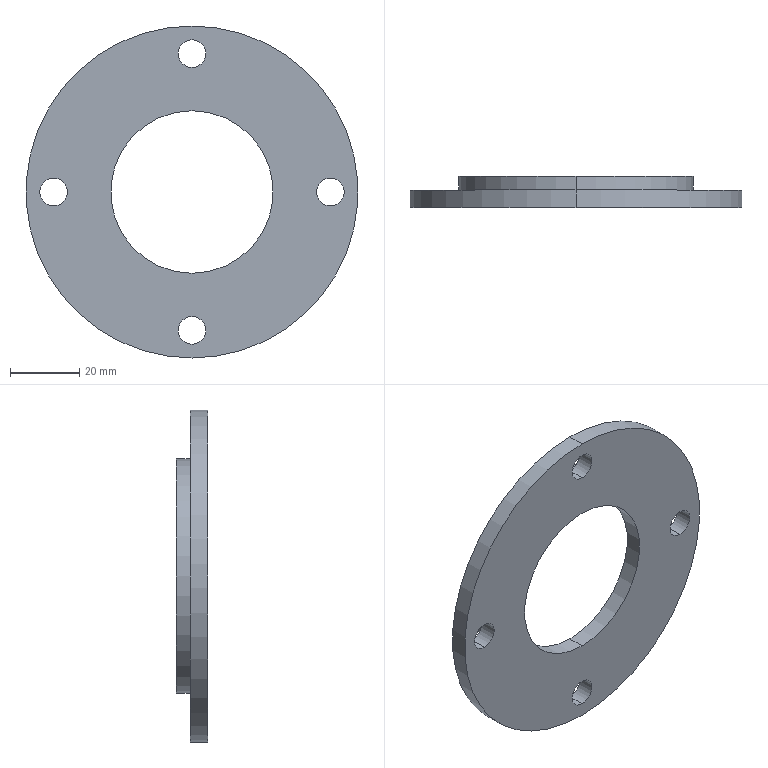Part | SolidWorks | features BaseBody 1 | 1 solid | 20 faces | box 96 x 9 x 96 mm | volume 29220 mm3 | cylinder 16 | plane 4 | commonest cylinder face diameters 8 x8 47 x2 61 x2 67.7 x2 96 x2
STEP:
#1=CARTESIAN_POINT('',(0.,5.,23.5));
#2=VERTEX_POINT('',#1);
#3=CARTESIAN_POINT('',(0.,5.,-23.5));
#4=VERTEX_POINT('',#3);
#5=CARTESIAN_POINT('',(0.,5.,0.));
#6=DIRECTION('',(0.,-1.,0.));
#7=DIRECTION('',(0.,0.,-1.));
#8=AXIS2_PLACEMENT_3D('',#5,#6,#7);
#9=CIRCLE('',#8,23.5);
#10=EDGE_CURVE('',#2,#4,#9,.T.);
#11=ORIENTED_EDGE('',*,*,#10,.F.);
#12=CARTESIAN_POINT('',(0.,0.,23.5));
#13=VERTEX_POINT('',#12);
#14=CARTESIAN_POINT('',(0.,5.,23.5));
#15=DIRECTION('',(0.,-1.,0.));
#16=VECTOR('',#15,1000.);
#17=LINE('',#14,#16);
#18=EDGE_CURVE('',#2,#13,#17,.T.);
#19=ORIENTED_EDGE('',*,*,#18,.T.);
#20=CARTESIAN_POINT('',(0.,0.,-23.5));
#21=VERTEX_POINT('',#20);
#22=CARTESIAN_POINT('',(0.,0.,0.));
#23=DIRECTION('',(0.,-1.,0.));
#24=DIRECTION('',(0.,0.,-1.));
#25=AXIS2_PLACEMENT_3D('',#22,#23,#24);
#26=CIRCLE('',#25,23.5);
#27=EDGE_CURVE('',#13,#21,#26,.T.);
#28=ORIENTED_EDGE('',*,*,#27,.T.);
#29=CARTESIAN_POINT('',(0.,5.,-23.5));
#30=DIRECTION('',(0.,-1.,0.));
#31=VECTOR('',#30,1000.);
#32=LINE('',#29,#31);
#33=EDGE_CURVE('',#4,#21,#32,.T.);
#34=ORIENTED_EDGE('',*,*,#33,.F.);
#35=EDGE_LOOP('',(#11,#19,#28,#34));
#36=FACE_OUTER_BOUND('',#35,.T.);
#37=CARTESIAN_POINT('',(0.,5.,0.));
#38=DIRECTION('',(0.,-1.,0.));
#39=DIRECTION('',(0.,0.,-1.));
#40=AXIS2_PLACEMENT_3D('',#37,#38,#39);
#41=CYLINDRICAL_SURFACE('',#40,23.5);
#42=ADVANCED_FACE('',(#36),#41,.F.);
#43=CARTESIAN_POINT('',(0.,5.,-48.));
#44=VERTEX_POINT('',#43);
#45=CARTESIAN_POINT('',(0.,5.,48.));
#46=VERTEX_POINT('',#45);
#47=CARTESIAN_POINT('',(0.,5.,0.));
#48=DIRECTION('',(0.,-1.,0.));
#49=DIRECTION('',(0.,0.,-1.));
#50=AXIS2_PLACEMENT_3D('',#47,#48,#49);
#51=CIRCLE('',#50,48.);
#52=EDGE_CURVE('',#44,#46,#51,.T.);
#53=ORIENTED_EDGE('',*,*,#52,.T.);
#54=CARTESIAN_POINT('',(0.,0.,48.));
#55=VERTEX_POINT('',#54);
#56=CARTESIAN_POINT('',(0.,5.,48.));
#57=DIRECTION('',(0.,-1.,0.));
#58=VECTOR('',#57,1000.);
#59=LINE('',#56,#58);
#60=EDGE_CURVE('',#46,#55,#59,.T.);
#61=ORIENTED_EDGE('',*,*,#60,.T.);
#62=CARTESIAN_POINT('',(0.,0.,-48.));
#63=VERTEX_POINT('',#62);
#64=CARTESIAN_POINT('',(0.,0.,0.));
#65=DIRECTION('',(0.,1.,0.));
#66=DIRECTION('',(0.,0.,-1.));
#67=AXIS2_PLACEMENT_3D('',#64,#65,#66);
#68=CIRCLE('',#67,48.);
#69=EDGE_CURVE('',#55,#63,#68,.T.);
#70=ORIENTED_EDGE('',*,*,#69,.T.);
#71=CARTESIAN_POINT('',(0.,5.,-48.));
#72=DIRECTION('',(0.,-1.,0.));
#73=VECTOR('',#72,1000.);
#74=LINE('',#71,#73);
#75=EDGE_CURVE('',#44,#63,#74,.T.);
#76=ORIENTED_EDGE('',*,*,#75,.F.);
#77=EDGE_LOOP('',(#53,#61,#70,#76));
#78=FACE_OUTER_BOUND('',#77,.T.);
#79=CARTESIAN_POINT('',(0.,5.,0.));
#80=DIRECTION('',(0.,-1.,0.));
#81=DIRECTION('',(0.,0.,-1.));
#82=AXIS2_PLACEMENT_3D('',#79,#80,#81);
#83=CYLINDRICAL_SURFACE('',#82,48.);
#84=ADVANCED_FACE('',(#78),#83,.T.);
#85=CARTESIAN_POINT('',(-40.,0.,4.));
#86=VERTEX_POINT('',#85);
#87=CARTESIAN_POINT('',(-40.,0.,-4.));
#88=VERTEX_POINT('',#87);
#89=CARTESIAN_POINT('',(-40.,0.,0.));
#90=DIRECTION('',(0.,-1.,0.));
#91=DIRECTION('',(0.,0.,1.));
#92=AXIS2_PLACEMENT_3D('',#89,#90,#91);
#93=CIRCLE('',#92,4.);
#94=EDGE_CURVE('',#86,#88,#93,.T.);
#95=ORIENTED_EDGE('',*,*,#94,.T.);
#96=CARTESIAN_POINT('',(-40.,5.,-4.));
#97=VERTEX_POINT('',#96);
#98=CARTESIAN_POINT('',(-40.,0.,-4.));
#99=DIRECTION('',(0.,1.,0.));
#100=VECTOR('',#99,1000.);
#101=LINE('',#98,#100);
#102=EDGE_CURVE('',#88,#97,#101,.T.);
#103=ORIENTED_EDGE('',*,*,#102,.T.);
#104=CARTESIAN_POINT('',(-40.,5.,4.));
#105=VERTEX_POINT('',#104);
#106=CARTESIAN_POINT('',(-40.,5.,0.));
#107=DIRECTION('',(0.,-1.,0.));
#108=DIRECTION('',(0.,0.,1.));
#109=AXIS2_PLACEMENT_3D('',#106,#107,#108);
#110=CIRCLE('',#109,4.);
#111=EDGE_CURVE('',#105,#97,#110,.T.);
#112=ORIENTED_EDGE('',*,*,#111,.F.);
#113=CARTESIAN_POINT('',(-40.,0.,4.));
#114=DIRECTION('',(0.,1.,0.));
#115=VECTOR('',#114,1000.);
#116=LINE('',#113,#115);
#117=EDGE_CURVE('',#86,#105,#116,.T.);
#118=ORIENTED_EDGE('',*,*,#117,.F.);
#119=EDGE_LOOP('',(#95,#103,#112,#118));
#120=FACE_OUTER_BOUND('',#119,.T.);
#121=CARTESIAN_POINT('',(-40.,0.,0.));
#122=DIRECTION('',(0.,1.,0.));
#123=DIRECTION('',(0.,0.,1.));
#124=AXIS2_PLACEMENT_3D('',#121,#122,#123);
#125=CYLINDRICAL_SURFACE('',#124,4.);
#126=ADVANCED_FACE('',(#120),#125,.F.);
#127=CARTESIAN_POINT('',(0.,0.,44.));
#128=VERTEX_POINT('',#127);
#129=CARTESIAN_POINT('',(0.,0.,36.));
#130=VERTEX_POINT('',#129);
#131=CARTESIAN_POINT('',(0.,0.,40.));
#132=DIRECTION('',(0.,-1.,0.));
#133=DIRECTION('',(0.,0.,1.));
#134=AXIS2_PLACEMENT_3D('',#131,#132,#133);
#135=CIRCLE('',#134,4.);
#136=EDGE_CURVE('',#128,#130,#135,.T.);
#137=ORIENTED_EDGE('',*,*,#136,.T.);
#138=CARTESIAN_POINT('',(0.,5.,36.));
#139=VERTEX_POINT('',#138);
#140=CARTESIAN_POINT('',(0.,0.,36.));
#141=DIRECTION('',(0.,1.,0.));
#142=VECTOR('',#141,1000.);
#143=LINE('',#140,#142);
#144=EDGE_CURVE('',#130,#139,#143,.T.);
#145=ORIENTED_EDGE('',*,*,#144,.T.);
#146=CARTESIAN_POINT('',(0.,5.,44.));
#147=VERTEX_POINT('',#146);
#148=CARTESIAN_POINT('',(0.,5.,40.));
#149=DIRECTION('',(0.,-1.,0.));
#150=DIRECTION('',(0.,0.,1.));
#151=AXIS2_PLACEMENT_3D('',#148,#149,#150);
#152=CIRCLE('',#151,4.);
#153=EDGE_CURVE('',#147,#139,#152,.T.);
#154=ORIENTED_EDGE('',*,*,#153,.F.);
#155=CARTESIAN_POINT('',(0.,0.,44.));
#156=DIRECTION('',(0.,1.,0.));
#157=VECTOR('',#156,1000.);
#158=LINE('',#155,#157);
#159=EDGE_CURVE('',#128,#147,#158,.T.);
#160=ORIENTED_EDGE('',*,*,#159,.F.);
#161=EDGE_LOOP('',(#137,#145,#154,#160));
#162=FACE_OUTER_BOUND('',#161,.T.);
#163=CARTESIAN_POINT('',(0.,0.,40.));
#164=DIRECTION('',(0.,1.,0.));
#165=DIRECTION('',(0.,0.,1.));
#166=AXIS2_PLACEMENT_3D('',#163,#164,#165);
#167=CYLINDRICAL_SURFACE('',#166,4.);
#168=ADVANCED_FACE('',(#162),#167,.F.);
#169=CARTESIAN_POINT('',(40.,0.,4.));
#170=VERTEX_POINT('',#169);
#171=CARTESIAN_POINT('',(40.,0.,-4.));
#172=VERTEX_POINT('',#171);
#173=CARTESIAN_POINT('',(40.,0.,0.));
#174=DIRECTION('',(0.,-1.,0.));
#175=DIRECTION('',(0.,0.,1.));
#176=AXIS2_PLACEMENT_3D('',#173,#174,#175);
#177=CIRCLE('',#176,4.);
#178=EDGE_CURVE('',#170,#172,#177,.T.);
#179=ORIENTED_EDGE('',*,*,#178,.T.);
#180=CARTESIAN_POINT('',(40.,5.,-4.));
#181=VERTEX_POINT('',#180);
#182=CARTESIAN_POINT('',(40.,0.,-4.));
#183=DIRECTION('',(0.,1.,0.));
#184=VECTOR('',#183,1000.);
#185=LINE('',#182,#184);
#186=EDGE_CURVE('',#172,#181,#185,.T.);
#187=ORIENTED_EDGE('',*,*,#186,.T.);
#188=CARTESIAN_POINT('',(40.,5.,4.));
#189=VERTEX_POINT('',#188);
#190=CARTESIAN_POINT('',(40.,5.,0.));
#191=DIRECTION('',(0.,-1.,0.));
#192=DIRECTION('',(0.,0.,1.));
#193=AXIS2_PLACEMENT_3D('',#190,#191,#192);
#194=CIRCLE('',#193,4.);
#195=EDGE_CURVE('',#189,#181,#194,.T.);
#196=ORIENTED_EDGE('',*,*,#195,.F.);
#197=CARTESIAN_POINT('',(40.,0.,4.));
#198=DIRECTION('',(0.,1.,0.));
#199=VECTOR('',#198,1000.);
#200=LINE('',#197,#199);
#201=EDGE_CURVE('',#170,#189,#200,.T.);
#202=ORIENTED_EDGE('',*,*,#201,.F.);
#203=EDGE_LOOP('',(#179,#187,#196,#202));
#204=FACE_OUTER_BOUND('',#203,.T.);
#205=CARTESIAN_POINT('',(40.,0.,0.));
#206=DIRECTION('',(0.,1.,0.));
#207=DIRECTION('',(0.,0.,1.));
#208=AXIS2_PLACEMENT_3D('',#205,#206,#207);
#209=CYLINDRICAL_SURFACE('',#208,4.);
#210=ADVANCED_FACE('',(#204),#209,.F.);
#211=CARTESIAN_POINT('',(0.,0.,-36.));
#212=VERTEX_POINT('',#211);
#213=CARTESIAN_POINT('',(0.,0.,-44.));
#214=VERTEX_POINT('',#213);
#215=CARTESIAN_POINT('',(0.,0.,-40.));
#216=DIRECTION('',(0.,-1.,0.));
#217=DIRECTION('',(0.,0.,1.));
#218=AXIS2_PLACEMENT_3D('',#215,#216,#217);
#219=CIRCLE('',#218,4.);
#220=EDGE_CURVE('',#212,#214,#219,.T.);
#221=ORIENTED_EDGE('',*,*,#220,.T.);
#222=CARTESIAN_POINT('',(0.,5.,-44.));
#223=VERTEX_POINT('',#222);
#224=CARTESIAN_POINT('',(0.,0.,-44.));
#225=DIRECTION('',(0.,1.,0.));
#226=VECTOR('',#225,1000.);
#227=LINE('',#224,#226);
#228=EDGE_CURVE('',#214,#223,#227,.T.);
#229=ORIENTED_EDGE('',*,*,#228,.T.);
#230=CARTESIAN_POINT('',(0.,5.,-36.));
#231=VERTEX_POINT('',#230);
#232=CARTESIAN_POINT('',(0.,5.,-40.));
#233=DIRECTION('',(0.,-1.,0.));
#234=DIRECTION('',(0.,0.,1.));
#235=AXIS2_PLACEMENT_3D('',#232,#233,#234);
#236=CIRCLE('',#235,4.);
#237=EDGE_CURVE('',#231,#223,#236,.T.);
#238=ORIENTED_EDGE('',*,*,#237,.F.);
#239=CARTESIAN_POINT('',(0.,0.,-36.));
#240=DIRECTION('',(0.,1.,0.));
#241=VECTOR('',#240,1000.);
#242=LINE('',#239,#241);
#243=EDGE_CURVE('',#212,#231,#242,.T.);
#244=ORIENTED_EDGE('',*,*,#243,.F.);
#245=EDGE_LOOP('',(#221,#229,#238,#244));
#246=FACE_OUTER_BOUND('',#245,.T.);
#247=CARTESIAN_POINT('',(0.,0.,-40.));
#248=DIRECTION('',(0.,1.,0.));
#249=DIRECTION('',(0.,0.,1.));
#250=AXIS2_PLACEMENT_3D('',#247,#248,#249);
#251=CYLINDRICAL_SURFACE('',#250,4.);
#252=ADVANCED_FACE('',(#246),#251,.F.);
#253=CARTESIAN_POINT('',(0.,9.,30.5));
#254=VERTEX_POINT('',#253);
#255=CARTESIAN_POINT('',(0.,9.,-30.5));
#256=VERTEX_POINT('',#255);
#257=CARTESIAN_POINT('',(0.,9.,0.));
#258=DIRECTION('',(0.,-1.,0.));
#259=DIRECTION('',(0.,0.,-1.));
#260=AXIS2_PLACEMENT_3D('',#257,#258,#259);
#261=CIRCLE('',#260,30.5);
#262=EDGE_CURVE('',#254,#256,#261,.T.);
#263=ORIENTED_EDGE('',*,*,#262,.F.);
#264=CARTESIAN_POINT('',(0.,5.,30.5));
#265=VERTEX_POINT('',#264);
#266=CARTESIAN_POINT('',(0.,9.,30.5));
#267=DIRECTION('',(0.,-1.,0.));
#268=VECTOR('',#267,1000.);
#269=LINE('',#266,#268);
#270=EDGE_CURVE('',#254,#265,#269,.T.);
#271=ORIENTED_EDGE('',*,*,#270,.T.);
#272=CARTESIAN_POINT('',(0.,5.,-30.5));
#273=VERTEX_POINT('',#272);
#274=CARTESIAN_POINT('',(0.,5.,0.));
#275=DIRECTION('',(0.,1.,0.));
#276=DIRECTION('',(0.,0.,-1.));
#277=AXIS2_PLACEMENT_3D('',#274,#275,#276);
#278=CIRCLE('',#277,30.5);
#279=EDGE_CURVE('',#273,#265,#278,.T.);
#280=ORIENTED_EDGE('',*,*,#279,.F.);
#281=CARTESIAN_POINT('',(0.,9.,-30.5));
#282=DIRECTION('',(0.,-1.,0.));
#283=VECTOR('',#282,1000.);
#284=LINE('',#281,#283);
#285=EDGE_CURVE('',#256,#273,#284,.T.);
#286=ORIENTED_EDGE('',*,*,#285,.F.);
#287=EDGE_LOOP('',(#263,#271,#280,#286));
#288=FACE_OUTER_BOUND('',#287,.T.);
#289=CARTESIAN_POINT('',(0.,9.,0.));
#290=DIRECTION('',(0.,-1.,0.));
#291=DIRECTION('',(0.,0.,-1.));
#292=AXIS2_PLACEMENT_3D('',#289,#290,#291);
#293=CYLINDRICAL_SURFACE('',#292,30.5);
#294=ADVANCED_FACE('',(#288),#293,.F.);
#295=CARTESIAN_POINT('',(0.,9.,-33.85));
#296=VERTEX_POINT('',#295);
#297=CARTESIAN_POINT('',(0.,9.,33.85));
#298=VERTEX_POINT('',#297);
#299=CARTESIAN_POINT('',(0.,9.,0.));
#300=DIRECTION('',(0.,-1.,0.));
#301=DIRECTION('',(0.,0.,-1.));
#302=AXIS2_PLACEMENT_3D('',#299,#300,#301);
#303=CIRCLE('',#302,33.85);
#304=EDGE_CURVE('',#296,#298,#303,.T.);
#305=ORIENTED_EDGE('',*,*,#304,.T.);
#306=CARTESIAN_POINT('',(0.,5.,33.85));
#307=VERTEX_POINT('',#306);
#308=CARTESIAN_POINT('',(0.,9.,33.85));
#309=DIRECTION('',(0.,-1.,0.));
#310=VECTOR('',#309,1000.);
#311=LINE('',#308,#310);
#312=EDGE_CURVE('',#298,#307,#311,.T.);
#313=ORIENTED_EDGE('',*,*,#312,.T.);
#314=CARTESIAN_POINT('',(0.,5.,-33.85));
#315=VERTEX_POINT('',#314);
#316=CARTESIAN_POINT('',(0.,5.,0.));
#317=DIRECTION('',(0.,-1.,0.));
#318=DIRECTION('',(0.,0.,-1.));
#319=AXIS2_PLACEMENT_3D('',#316,#317,#318);
#320=CIRCLE('',#319,33.85);
#321=EDGE_CURVE('',#315,#307,#320,.T.);
#322=ORIENTED_EDGE('',*,*,#321,.F.);
#323=CARTESIAN_POINT('',(0.,9.,-33.85));
#324=DIRECTION('',(0.,-1.,0.));
#325=VECTOR('',#324,1000.);
#326=LINE('',#323,#325);
#327=EDGE_CURVE('',#296,#315,#326,.T.);
#328=ORIENTED_EDGE('',*,*,#327,.F.);
#329=EDGE_LOOP('',(#305,#313,#322,#328));
#330=FACE_OUTER_BOUND('',#329,.T.);
#331=CARTESIAN_POINT('',(0.,9.,0.));
#332=DIRECTION('',(0.,-1.,0.));
#333=DIRECTION('',(0.,0.,-1.));
#334=AXIS2_PLACEMENT_3D('',#331,#332,#333);
#335=CYLINDRICAL_SURFACE('',#334,33.85);
#336=ADVANCED_FACE('',(#330),#335,.T.);
#337=CARTESIAN_POINT('',(0.,0.,0.));
#338=DIRECTION('',(0.,-1.,0.));
#339=DIRECTION('',(0.,0.,-1.));
#340=AXIS2_PLACEMENT_3D('',#337,#338,#339);
#341=CIRCLE('',#340,23.5);
#342=EDGE_CURVE('',#21,#13,#341,.T.);
#343=ORIENTED_EDGE('',*,*,#342,.F.);
#344=ORIENTED_EDGE('',*,*,#27,.F.);
#345=EDGE_LOOP('',(#343,#344));
#346=FACE_BOUND('',#345,.T.);
#347=CARTESIAN_POINT('',(0.,0.,0.));
#348=DIRECTION('',(0.,1.,0.));
#349=DIRECTION('',(0.,0.,-1.));
#350=AXIS2_PLACEMENT_3D('',#347,#348,#349);
#351=CIRCLE('',#350,48.);
#352=EDGE_CURVE('',#63,#55,#351,.T.);
#353=ORIENTED_EDGE('',*,*,#352,.F.);
#354=ORIENTED_EDGE('',*,*,#69,.F.);
#355=EDGE_LOOP('',(#353,#354));
#356=FACE_OUTER_BOUND('',#355,.T.);
#357=ORIENTED_EDGE('',*,*,#94,.F.);
#358=CARTESIAN_POINT('',(-40.,0.,0.));
#359=DIRECTION('',(0.,-1.,0.));
#360=DIRECTION('',(0.,0.,1.));
#361=AXIS2_PLACEMENT_3D('',#358,#359,#360);
#362=CIRCLE('',#361,4.);
#363=EDGE_CURVE('',#88,#86,#362,.T.);
#364=ORIENTED_EDGE('',*,*,#363,.F.);
#365=EDGE_LOOP('',(#357,#364));
#366=FACE_BOUND('',#365,.T.);
#367=ORIENTED_EDGE('',*,*,#136,.F.);
#368=CARTESIAN_POINT('',(0.,0.,40.));
#369=DIRECTION('',(0.,-1.,0.));
#370=DIRECTION('',(0.,0.,1.));
#371=AXIS2_PLACEMENT_3D('',#368,#369,#370);
#372=CIRCLE('',#371,4.);
#373=EDGE_CURVE('',#130,#128,#372,.T.);
#374=ORIENTED_EDGE('',*,*,#373,.F.);
#375=EDGE_LOOP('',(#367,#374));
#376=FACE_BOUND('',#375,.T.);
#377=ORIENTED_EDGE('',*,*,#178,.F.);
#378=CARTESIAN_POINT('',(40.,0.,0.));
#379=DIRECTION('',(0.,-1.,0.));
#380=DIRECTION('',(0.,0.,1.));
#381=AXIS2_PLACEMENT_3D('',#378,#379,#380);
#382=CIRCLE('',#381,4.);
#383=EDGE_CURVE('',#172,#170,#382,.T.);
#384=ORIENTED_EDGE('',*,*,#383,.F.);
#385=EDGE_LOOP('',(#377,#384));
#386=FACE_BOUND('',#385,.T.);
#387=ORIENTED_EDGE('',*,*,#220,.F.);
#388=CARTESIAN_POINT('',(0.,0.,-40.));
#389=DIRECTION('',(0.,-1.,0.));
#390=DIRECTION('',(0.,0.,1.));
#391=AXIS2_PLACEMENT_3D('',#388,#389,#390);
#392=CIRCLE('',#391,4.);
#393=EDGE_CURVE('',#214,#212,#392,.T.);
#394=ORIENTED_EDGE('',*,*,#393,.F.);
#395=EDGE_LOOP('',(#387,#394));
#396=FACE_BOUND('',#395,.T.);
#397=CARTESIAN_POINT('',(0.,0.,0.));
#398=DIRECTION('',(0.,1.,0.));
#399=DIRECTION('',(0.,0.,1.));
#400=AXIS2_PLACEMENT_3D('',#397,#398,#399);
#401=PLANE('',#400);
#402=ADVANCED_FACE('',(#346,#356,#366,#376,#386,#396),#401,.F.);
#403=ORIENTED_EDGE('',*,*,#18,.F.);
#404=CARTESIAN_POINT('',(0.,5.,0.));
#405=DIRECTION('',(0.,-1.,0.));
#406=DIRECTION('',(0.,0.,-1.));
#407=AXIS2_PLACEMENT_3D('',#404,#405,#406);
#408=CIRCLE('',#407,23.5);
#409=EDGE_CURVE('',#4,#2,#408,.T.);
#410=ORIENTED_EDGE('',*,*,#409,.F.);
#411=ORIENTED_EDGE('',*,*,#33,.T.);
#412=ORIENTED_EDGE('',*,*,#342,.T.);
#413=EDGE_LOOP('',(#403,#410,#411,#412));
#414=FACE_OUTER_BOUND('',#413,.T.);
#415=CARTESIAN_POINT('',(0.,5.,0.));
#416=DIRECTION('',(0.,-1.,0.));
#417=DIRECTION('',(0.,0.,-1.));
#418=AXIS2_PLACEMENT_3D('',#415,#416,#417);
#419=CYLINDRICAL_SURFACE('',#418,23.5);
#420=ADVANCED_FACE('',(#414),#419,.F.);
#421=ORIENTED_EDGE('',*,*,#60,.F.);
#422=CARTESIAN_POINT('',(0.,5.,0.));
#423=DIRECTION('',(0.,-1.,0.));
#424=DIRECTION('',(0.,0.,-1.));
#425=AXIS2_PLACEMENT_3D('',#422,#423,#424);
#426=CIRCLE('',#425,48.);
#427=EDGE_CURVE('',#46,#44,#426,.T.);
#428=ORIENTED_EDGE('',*,*,#427,.T.);
#429=ORIENTED_EDGE('',*,*,#75,.T.);
#430=ORIENTED_EDGE('',*,*,#352,.T.);
#431=EDGE_LOOP('',(#421,#428,#429,#430));
#432=FACE_OUTER_BOUND('',#431,.T.);
#433=CARTESIAN_POINT('',(0.,5.,0.));
#434=DIRECTION('',(0.,-1.,0.));
#435=DIRECTION('',(0.,0.,-1.));
#436=AXIS2_PLACEMENT_3D('',#433,#434,#435);
#437=CYLINDRICAL_SURFACE('',#436,48.);
#438=ADVANCED_FACE('',(#432),#437,.T.);
#439=ORIENTED_EDGE('',*,*,#102,.F.);
#440=ORIENTED_EDGE('',*,*,#363,.T.);
#441=ORIENTED_EDGE('',*,*,#117,.T.);
#442=CARTESIAN_POINT('',(-40.,5.,0.));
#443=DIRECTION('',(0.,-1.,0.));
#444=DIRECTION('',(0.,0.,1.));
#445=AXIS2_PLACEMENT_3D('',#442,#443,#444);
#446=CIRCLE('',#445,4.);
#447=EDGE_CURVE('',#97,#105,#446,.T.);
#448=ORIENTED_EDGE('',*,*,#447,.F.);
#449=EDGE_LOOP('',(#439,#440,#441,#448));
#450=FACE_OUTER_BOUND('',#449,.T.);
#451=CARTESIAN_POINT('',(-40.,0.,0.));
#452=DIRECTION('',(0.,1.,0.));
#453=DIRECTION('',(0.,0.,1.));
#454=AXIS2_PLACEMENT_3D('',#451,#452,#453);
#455=CYLINDRICAL_SURFACE('',#454,4.);
#456=ADVANCED_FACE('',(#450),#455,.F.);
#457=ORIENTED_EDGE('',*,*,#144,.F.);
#458=ORIENTED_EDGE('',*,*,#373,.T.);
#459=ORIENTED_EDGE('',*,*,#159,.T.);
#460=CARTESIAN_POINT('',(0.,5.,40.));
#461=DIRECTION('',(0.,-1.,0.));
#462=DIRECTION('',(0.,0.,1.));
#463=AXIS2_PLACEMENT_3D('',#460,#461,#462);
#464=CIRCLE('',#463,4.);
#465=EDGE_CURVE('',#139,#147,#464,.T.);
#466=ORIENTED_EDGE('',*,*,#465,.F.);
#467=EDGE_LOOP('',(#457,#458,#459,#466));
#468=FACE_OUTER_BOUND('',#467,.T.);
#469=CARTESIAN_POINT('',(0.,0.,40.));
#470=DIRECTION('',(0.,1.,0.));
#471=DIRECTION('',(0.,0.,1.));
#472=AXIS2_PLACEMENT_3D('',#469,#470,#471);
#473=CYLINDRICAL_SURFACE('',#472,4.);
#474=ADVANCED_FACE('',(#468),#473,.F.);
#475=ORIENTED_EDGE('',*,*,#186,.F.);
#476=ORIENTED_EDGE('',*,*,#383,.T.);
#477=ORIENTED_EDGE('',*,*,#201,.T.);
#478=CARTESIAN_POINT('',(40.,5.,0.));
#479=DIRECTION('',(0.,-1.,0.));
#480=DIRECTION('',(0.,0.,1.));
#481=AXIS2_PLACEMENT_3D('',#478,#479,#480);
#482=CIRCLE('',#481,4.);
#483=EDGE_CURVE('',#181,#189,#482,.T.);
#484=ORIENTED_EDGE('',*,*,#483,.F.);
#485=EDGE_LOOP('',(#475,#476,#477,#484));
#486=FACE_OUTER_BOUND('',#485,.T.);
#487=CARTESIAN_POINT('',(40.,0.,0.));
#488=DIRECTION('',(0.,1.,0.));
#489=DIRECTION('',(0.,0.,1.));
#490=AXIS2_PLACEMENT_3D('',#487,#488,#489);
#491=CYLINDRICAL_SURFACE('',#490,4.);
#492=ADVANCED_FACE('',(#486),#491,.F.);
#493=ORIENTED_EDGE('',*,*,#228,.F.);
#494=ORIENTED_EDGE('',*,*,#393,.T.);
#495=ORIENTED_EDGE('',*,*,#243,.T.);
#496=CARTESIAN_POINT('',(0.,5.,-40.));
#497=DIRECTION('',(0.,-1.,0.));
#498=DIRECTION('',(0.,0.,1.));
#499=AXIS2_PLACEMENT_3D('',#496,#497,#498);
#500=CIRCLE('',#499,4.);
#501=EDGE_CURVE('',#223,#231,#500,.T.);
#502=ORIENTED_EDGE('',*,*,#501,.F.);
#503=EDGE_LOOP('',(#493,#494,#495,#502));
#504=FACE_OUTER_BOUND('',#503,.T.);
#505=CARTESIAN_POINT('',(0.,0.,-40.));
#506=DIRECTION('',(0.,1.,0.));
#507=DIRECTION('',(0.,0.,1.));
#508=AXIS2_PLACEMENT_3D('',#505,#506,#507);
#509=CYLINDRICAL_SURFACE('',#508,4.);
#510=ADVANCED_FACE('',(#504),#509,.F.);
#511=ORIENTED_EDGE('',*,*,#279,.T.);
#512=CARTESIAN_POINT('',(0.,5.,0.));
#513=DIRECTION('',(0.,1.,0.));
#514=DIRECTION('',(0.,0.,-1.));
#515=AXIS2_PLACEMENT_3D('',#512,#513,#514);
#516=CIRCLE('',#515,30.5);
#517=EDGE_CURVE('',#265,#273,#516,.T.);
#518=ORIENTED_EDGE('',*,*,#517,.T.);
#519=EDGE_LOOP('',(#511,#518));
#520=FACE_OUTER_BOUND('',#519,.T.);
#521=ORIENTED_EDGE('',*,*,#409,.T.);
#522=ORIENTED_EDGE('',*,*,#10,.T.);
#523=EDGE_LOOP('',(#521,#522));
#524=FACE_BOUND('',#523,.T.);
#525=CARTESIAN_POINT('',(0.,5.,0.));
#526=DIRECTION('',(0.,1.,0.));
#527=DIRECTION('',(0.,0.,1.));
#528=AXIS2_PLACEMENT_3D('',#525,#526,#527);
#529=PLANE('',#528);
#530=ADVANCED_FACE('',(#520,#524),#529,.T.);
#531=ORIENTED_EDGE('',*,*,#52,.F.);
#532=ORIENTED_EDGE('',*,*,#427,.F.);
#533=EDGE_LOOP('',(#531,#532));
#534=FACE_OUTER_BOUND('',#533,.T.);
#535=ORIENTED_EDGE('',*,*,#321,.T.);
#536=CARTESIAN_POINT('',(0.,5.,0.));
#537=DIRECTION('',(0.,-1.,0.));
#538=DIRECTION('',(0.,0.,-1.));
#539=AXIS2_PLACEMENT_3D('',#536,#537,#538);
#540=CIRCLE('',#539,33.85);
#541=EDGE_CURVE('',#307,#315,#540,.T.);
#542=ORIENTED_EDGE('',*,*,#541,.T.);
#543=EDGE_LOOP('',(#535,#542));
#544=FACE_BOUND('',#543,.T.);
#545=ORIENTED_EDGE('',*,*,#111,.T.);
#546=ORIENTED_EDGE('',*,*,#447,.T.);
#547=EDGE_LOOP('',(#545,#546));
#548=FACE_BOUND('',#547,.T.);
#549=ORIENTED_EDGE('',*,*,#153,.T.);
#550=ORIENTED_EDGE('',*,*,#465,.T.);
#551=EDGE_LOOP('',(#549,#550));
#552=FACE_BOUND('',#551,.T.);
#553=ORIENTED_EDGE('',*,*,#195,.T.);
#554=ORIENTED_EDGE('',*,*,#483,.T.);
#555=EDGE_LOOP('',(#553,#554));
#556=FACE_BOUND('',#555,.T.);
#557=ORIENTED_EDGE('',*,*,#237,.T.);
#558=ORIENTED_EDGE('',*,*,#501,.T.);
#559=EDGE_LOOP('',(#557,#558));
#560=FACE_BOUND('',#559,.T.);
#561=CARTESIAN_POINT('',(0.,5.,0.));
#562=DIRECTION('',(0.,1.,0.));
#563=DIRECTION('',(0.,0.,1.));
#564=AXIS2_PLACEMENT_3D('',#561,#562,#563);
#565=PLANE('',#564);
#566=ADVANCED_FACE('',(#534,#544,#548,#552,#556,#560),#565,.T.);
#567=ORIENTED_EDGE('',*,*,#270,.F.);
#568=CARTESIAN_POINT('',(0.,9.,0.));
#569=DIRECTION('',(0.,-1.,0.));
#570=DIRECTION('',(0.,0.,-1.));
#571=AXIS2_PLACEMENT_3D('',#568,#569,#570);
#572=CIRCLE('',#571,30.5);
#573=EDGE_CURVE('',#256,#254,#572,.T.);
#574=ORIENTED_EDGE('',*,*,#573,.F.);
#575=ORIENTED_EDGE('',*,*,#285,.T.);
#576=ORIENTED_EDGE('',*,*,#517,.F.);
#577=EDGE_LOOP('',(#567,#574,#575,#576));
#578=FACE_OUTER_BOUND('',#577,.T.);
#579=CARTESIAN_POINT('',(0.,9.,0.));
#580=DIRECTION('',(0.,-1.,0.));
#581=DIRECTION('',(0.,0.,-1.));
#582=AXIS2_PLACEMENT_3D('',#579,#580,#581);
#583=CYLINDRICAL_SURFACE('',#582,30.5);
#584=ADVANCED_FACE('',(#578),#583,.F.);
#585=ORIENTED_EDGE('',*,*,#312,.F.);
#586=CARTESIAN_POINT('',(0.,9.,0.));
#587=DIRECTION('',(0.,-1.,0.));
#588=DIRECTION('',(0.,0.,-1.));
#589=AXIS2_PLACEMENT_3D('',#586,#587,#588);
#590=CIRCLE('',#589,33.85);
#591=EDGE_CURVE('',#298,#296,#590,.T.);
#592=ORIENTED_EDGE('',*,*,#591,.T.);
#593=ORIENTED_EDGE('',*,*,#327,.T.);
#594=ORIENTED_EDGE('',*,*,#541,.F.);
#595=EDGE_LOOP('',(#585,#592,#593,#594));
#596=FACE_OUTER_BOUND('',#595,.T.);
#597=CARTESIAN_POINT('',(0.,9.,0.));
#598=DIRECTION('',(0.,-1.,0.));
#599=DIRECTION('',(0.,0.,-1.));
#600=AXIS2_PLACEMENT_3D('',#597,#598,#599);
#601=CYLINDRICAL_SURFACE('',#600,33.85);
#602=ADVANCED_FACE('',(#596),#601,.T.);
#603=ORIENTED_EDGE('',*,*,#573,.T.);
#604=ORIENTED_EDGE('',*,*,#262,.T.);
#605=EDGE_LOOP('',(#603,#604));
#606=FACE_BOUND('',#605,.T.);
#607=ORIENTED_EDGE('',*,*,#304,.F.);
#608=ORIENTED_EDGE('',*,*,#591,.F.);
#609=EDGE_LOOP('',(#607,#608));
#610=FACE_OUTER_BOUND('',#609,.T.);
#611=CARTESIAN_POINT('',(0.,9.,0.));
#612=DIRECTION('',(0.,1.,0.));
#613=DIRECTION('',(0.,0.,1.));
#614=AXIS2_PLACEMENT_3D('',#611,#612,#613);
#615=PLANE('',#614);
#616=ADVANCED_FACE('',(#606,#610),#615,.T.);
#617=CLOSED_SHELL('',(#42,#84,#126,#168,#210,#252,#294,#336,#402,#420,#438,#456,#474,#492,#510,#530,#566,#584,#602,#616));
#618=MANIFOLD_SOLID_BREP('',#617);
#619=CARTESIAN_POINT('',(0.,0.,0.));
#620=DIRECTION('',(0.,0.,1.));
#621=DIRECTION('',(1.,0.,0.));
#622=AXIS2_PLACEMENT_3D('',#619,#620,#621);
#623=(LENGTH_UNIT()NAMED_UNIT(*)SI_UNIT(.MILLI.,.METRE.));
#624=UNCERTAINTY_MEASURE_WITH_UNIT(LENGTH_MEASURE(0.00001),#623,'','');
#625=(NAMED_UNIT(*)PLANE_ANGLE_UNIT()SI_UNIT($,.RADIAN.));
#626=(NAMED_UNIT(*)SI_UNIT($,.STERADIAN.)SOLID_ANGLE_UNIT());
#627=(GEOMETRIC_REPRESENTATION_CONTEXT(3)GLOBAL_UNCERTAINTY_ASSIGNED_CONTEXT((#624))GLOBAL_UNIT_ASSIGNED_CONTEXT((#623,#625,#626))REPRESENTATION_CONTEXT('',''));
#628=ADVANCED_BREP_SHAPE_REPRESENTATION('',(#618,#622),#627);